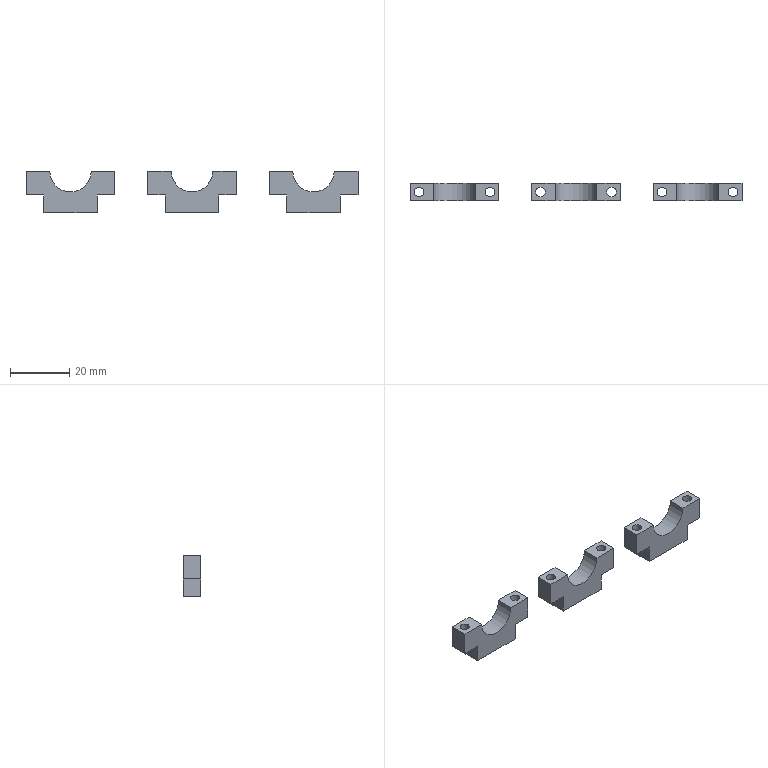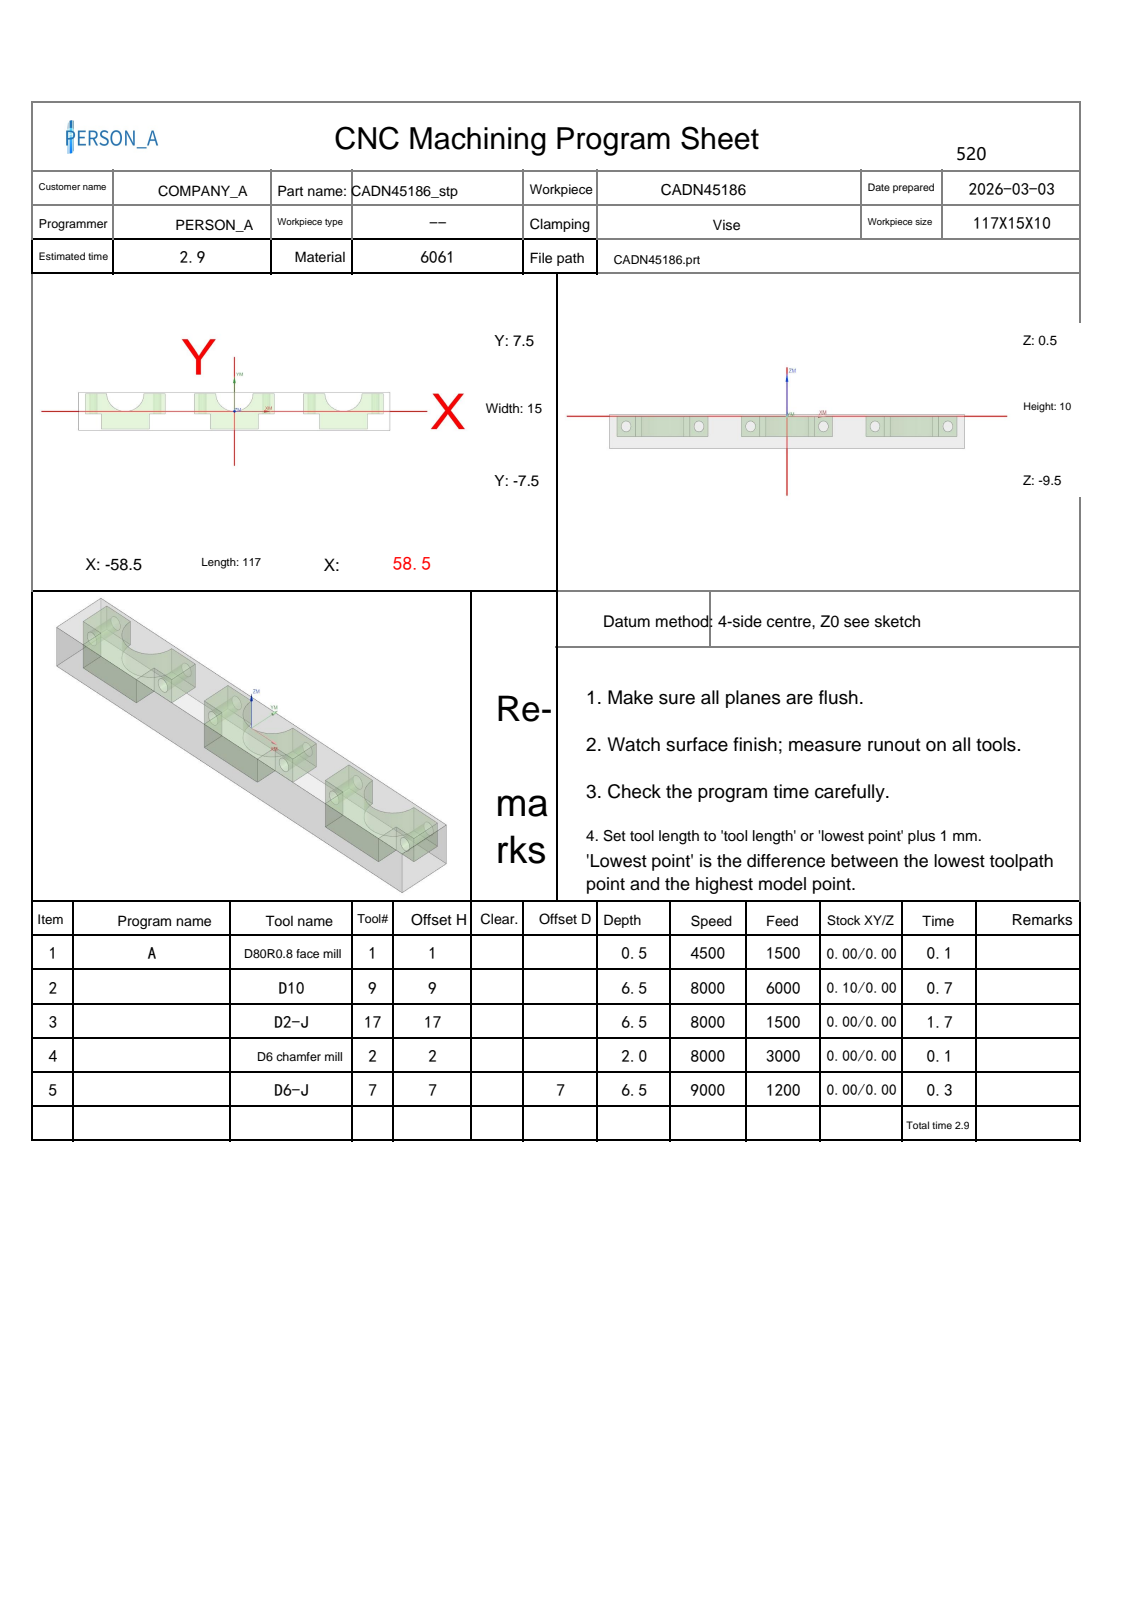NC program | NX | posted by the shop | part box 112 x 6 x 14 mm
Lines 1 to 633 of 5059:
%
O0001
(Machine time: 3.93 MIN)
(===Total Tool:5===)
(T1=D80R0.8 face mill D=80.  R=0.8  D-  H01 Z=0.    )
(T9=D10     D=10.  R=0.   D-  H09 Z=-6.   )
(T17=D2-J   D=2.   R=0.   D-  H17 Z=-6.   )
(T2=D6 chamfer mill   D=6.   R=0.   D-  H02 Z=-1.5  )
(T7=D6-J    D=6.   R=0.   D7  H07 Z=-6.   )
G80 G90 G17 G49 G40
G91 G28 Z0
M01
N1 T01 M06
(D80R0.8 face mill  D=80. R=0.8 H=01 ce=0.00 di=0.00)
(MAX_Z=50. MIN_Z=0. Time=0.15M)
G00 G90 G54 X101. Y0.0 M03 S4500
G43 H01 Z50.
M08
Z2.
G01 Z0.0 F1500.
X96.
X-96.
X-101.
Z2.
G00 Z50.
G91 G28 Z0.0
M05
M09
G91 G28 Z0.0
M01
N2 T09 M06
(D10  D=10. R=0. H=09 ce=0.10 di=0.00)
(MAX_Z=50. MIN_Z=-6. Time=0.65M)
G00 G90 G54 X41. Y-12.1 M03 S8000
G43 H09 Z50.
M08
Z.5
G01 X32. Z.447 F6000.
G02 X26.9 Y-7. Z.401 I0.0 J5.1
G01 Y-6.1 Z.395
X26. Z.39
G02 X20.9 Y-1. Z.343 I0.0 J5.1
G01 Y7. Z.297
G02 X26. Y12.1 Z.25 I5.1 J0.0
G01 X34. Z.203
G02 X39.1 Y7. Z.156 I0.0 J-5.1
G03 X41. Y5.1 Z.139 I1.9 J0.0
X42.9 Y7. Z.121 I0.0 J1.9
G02 X48. Y12.1 Z.075 I5.1 J0.0
G01 X56. Z.028
G02 X61.1 Y7. Z-.019 I0.0 J-5.1
G01 Y-1. Z-.066
G02 X56. Y-6.1 Z-.112 I-5.1 J0.0
G01 X55.1 Z-.118
Y-7. Z-.123
G02 X50. Y-12.1 Z-.17 I-5.1 J0.0
G01 X32. Z-.275
G02 X26.9 Y-7. Z-.322 I0.0 J5.1
G01 Y-6.1 Z-.327
X26. Z-.332
G02 X20.9 Y-1. Z-.379 I0.0 J5.1
G01 Y7. Z-.426
G02 X26. Y12.1 Z-.472 I5.1 J0.0
G01 X34. Z-.519
G02 X39.1 Y7. Z-.566 I0.0 J-5.1
G03 X41. Y5.1 Z-.583 I1.9 J0.0
X42.9 Y7. Z-.601 I0.0 J1.9
G02 X48. Y12.1 Z-.648 I5.1 J0.0
G01 X56. Z-.694
G02 X61.1 Y7. Z-.741 I0.0 J-5.1
G01 Y-1. Z-.788
G02 X56. Y-6.1 Z-.835 I-5.1 J0.0
G01 X55.1 Z-.84
Y-7. Z-.845
G02 X50. Y-12.1 Z-.892 I-5.1 J0.0
G01 X32. Z-.997
G02 X26.9 Y-7. Z-1.044 I0.0 J5.1
G01 Y-6.1 Z-1.049
X26. Z-1.054
G02 X20.9 Y-1. Z-1.101 I0.0 J5.1
G01 Y7. Z-1.148
G02 X26. Y12.1 Z-1.195 I5.1 J0.0
G01 X34. Z-1.241
G02 X39.1 Y7. Z-1.288 I0.0 J-5.1
G03 X41. Y5.1 Z-1.306 I1.9 J0.0
X42.9 Y7. Z-1.323 I0.0 J1.9
G02 X48. Y12.1 Z-1.37 I5.1 J0.0
G01 X56. Z-1.417
G02 X61.1 Y7. Z-1.463 I0.0 J-5.1
G01 Y-1. Z-1.51
G02 X56. Y-6.1 Z-1.557 I-5.1 J0.0
G01 X55.1 Z-1.562
Y-7. Z-1.567
G02 X50. Y-12.1 Z-1.614 I-5.1 J0.0
G01 X32. Z-1.719
G02 X26.9 Y-7. Z-1.766 I0.0 J5.1
G01 Y-6.1 Z-1.771
X26. Z-1.777
G02 X20.9 Y-1. Z-1.823 I0.0 J5.1
G01 Y7. Z-1.87
G02 X26. Y12.1 Z-1.917 I5.1 J0.0
G01 X34. Z-1.964
G02 X39.1 Y7. Z-2.01 I0.0 J-5.1
G03 X41. Y5.1 Z-2.028 I1.9 J0.0
X42.9 Y7. Z-2.045 I0.0 J1.9
G02 X48. Y12.1 Z-2.092 I5.1 J0.0
G01 X56. Z-2.139
G02 X61.1 Y7. Z-2.186 I0.0 J-5.1
G01 Y-1. Z-2.232
G02 X56. Y-6.1 Z-2.279 I-5.1 J0.0
G01 X55.1 Z-2.284
Y-7. Z-2.29
G02 X50. Y-12.1 Z-2.336 I-5.1 J0.0
G01 X32. Z-2.441
G02 X26.9 Y-7. Z-2.488 I0.0 J5.1
G01 Y-6.1 Z-2.493
X26. Z-2.499
G02 X20.9 Y-1. Z-2.546 I0.0 J5.1
G01 Y7. Z-2.592
G02 X26. Y12.1 Z-2.639 I5.1 J0.0
G01 X34. Z-2.686
G02 X39.1 Y7. Z-2.733 I0.0 J-5.1
G03 X41. Y5.1 Z-2.75 I1.9 J0.0
X42.9 Y7. Z-2.767 I0.0 J1.9
G02 X48. Y12.1 Z-2.814 I5.1 J0.0
G01 X56. Z-2.861
G02 X61.1 Y7. Z-2.908 I0.0 J-5.1
G01 Y-1. Z-2.954
G02 X56. Y-6.1 Z-3.001 I-5.1 J0.0
G01 X55.1 Z-3.007
Y-7. Z-3.012
G02 X50. Y-12.1 Z-3.059 I-5.1 J0.0
G01 X32. Z-3.164
G02 X26.9 Y-7. Z-3.21 I0.0 J5.1
G01 Y-6.1 Z-3.216
X26. Z-3.221
G02 X20.9 Y-1. Z-3.268 I0.0 J5.1
G01 Y7. Z-3.314
G02 X26. Y12.1 Z-3.361 I5.1 J0.0
G01 X34. Z-3.408
G02 X39.1 Y7. Z-3.455 I0.0 J-5.1
G03 X41. Y5.1 Z-3.472 I1.9 J0.0
X42.9 Y7. Z-3.49 I0.0 J1.9
G02 X48. Y12.1 Z-3.536 I5.1 J0.0
G01 X56. Z-3.583
G02 X61.1 Y7. Z-3.63 I0.0 J-5.1
G01 Y-1. Z-3.677
G02 X56. Y-6.1 Z-3.723 I-5.1 J0.0
G01 X55.1 Z-3.729
Y-7. Z-3.734
G02 X50. Y-12.1 Z-3.781 I-5.1 J0.0
G01 X32. Z-3.886
G02 X26.9 Y-7. Z-3.933 I0.0 J5.1
G01 Y-6.1 Z-3.938
X26. Z-3.943
G02 X20.9 Y-1. Z-3.99 I0.0 J5.1
G01 Y7. Z-4.037
G02 X26. Y12.1 Z-4.084 I5.1 J0.0
G01 X34. Z-4.13
G02 X39.1 Y7. Z-4.177 I0.0 J-5.1
G03 X41. Y5.1 Z-4.194 I1.9 J0.0
X42.9 Y7. Z-4.212 I0.0 J1.9
G02 X48. Y12.1 Z-4.259 I5.1 J0.0
G01 X56. Z-4.305
G02 X61.1 Y7. Z-4.352 I0.0 J-5.1
G01 Y-1. Z-4.399
G02 X56. Y-6.1 Z-4.446 I-5.1 J0.0
G01 X55.1 Z-4.451
Y-7. Z-4.456
G02 X50. Y-12.1 Z-4.503 I-5.1 J0.0
G01 X32. Z-4.608
G02 X26.9 Y-7. Z-4.655 I0.0 J5.1
G01 Y-6.1 Z-4.66
X26. Z-4.665
G02 X20.9 Y-1. Z-4.712 I0.0 J5.1
G01 Y7. Z-4.759
G02 X26. Y12.1 Z-4.806 I5.1 J0.0
G01 X34. Z-4.852
G02 X39.1 Y7. Z-4.899 I0.0 J-5.1
G03 X41. Y5.1 Z-4.917 I1.9 J0.0
X42.9 Y7. Z-4.934 I0.0 J1.9
G02 X48. Y12.1 Z-4.981 I5.1 J0.0
G01 X56. Z-5.028
G02 X61.1 Y7. Z-5.074 I0.0 J-5.1
G01 Y-1. Z-5.121
G02 X56. Y-6.1 Z-5.168 I-5.1 J0.0
G01 X55.1 Z-5.173
Y-7. Z-5.178
G02 X50. Y-12.1 Z-5.225 I-5.1 J0.0
G01 X32. Z-5.33
G02 X26.9 Y-7. Z-5.377 I0.0 J5.1
G01 Y-6.1 Z-5.382
X26. Z-5.388
G02 X20.9 Y-1. Z-5.434 I0.0 J5.1
G01 Y7. Z-5.481
G02 X26. Y12.1 Z-5.528 I5.1 J0.0
G01 X34. Z-5.575
G02 X39.1 Y7. Z-5.621 I0.0 J-5.1
G03 X41. Y5.1 Z-5.639 I1.9 J0.0
X42.9 Y7. Z-5.656 I0.0 J1.9
G02 X48. Y12.1 Z-5.703 I5.1 J0.0
G01 X56. Z-5.75
G02 X61.1 Y7. Z-5.797 I0.0 J-5.1
G01 Y-1. Z-5.843
G02 X56. Y-6.1 Z-5.89 I-5.1 J0.0
G01 X55.1 Z-5.895
Y-7. Z-5.901
G02 X50. Y-12.1 Z-5.947 I-5.1 J0.0
G01 X41. Z-6.
X32.
G02 X26.9 Y-7. I0.0 J5.1
G01 Y-6.1
X26.
G02 X20.9 Y-1. I0.0 J5.1
G01 Y7.
G02 X26. Y12.1 I5.1 J0.0
G01 X34.
G02 X39.1 Y7. I0.0 J-5.1
G03 X41. Y5.1 I1.9 J0.0
X42.9 Y7. I0.0 J1.9
G02 X48. Y12.1 I5.1 J0.0
G01 X56.
G02 X61.1 Y7. I0.0 J-5.1
G01 Y-1.
G02 X56. Y-6.1 I-5.1 J0.0
G01 X55.1
Y-7.
G02 X50. Y-12.1 I-5.1 J0.0
G01 X41.
X40.5
Z-5.
G00 Z50.
X0.0
Z.5
G01 X-9. Z.447
G02 X-14.1 Y-7. Z.401 I0.0 J5.1
G01 Y-6.1 Z.395
X-15. Z.39
G02 X-20.1 Y-1. Z.343 I0.0 J5.1
G01 Y7. Z.297
G02 X-15. Y12.1 Z.25 I5.1 J0.0
G01 X-7. Z.203
G02 X-1.9 Y7. Z.156 I0.0 J-5.1
G03 X0.0 Y5.1 Z.139 I1.9 J0.0
X1.9 Y7. Z.121 I0.0 J1.9
G02 X7. Y12.1 Z.075 I5.1 J0.0
G01 X15. Z.028
G02 X20.1 Y7. Z-.019 I0.0 J-5.1
G01 Y-1. Z-.066
G02 X15. Y-6.1 Z-.112 I-5.1 J0.0
G01 X14.1 Z-.118
Y-7. Z-.123
G02 X9. Y-12.1 Z-.17 I-5.1 J0.0
G01 X-9. Z-.275
G02 X-14.1 Y-7. Z-.322 I0.0 J5.1
G01 Y-6.1 Z-.327
X-15. Z-.332
G02 X-20.1 Y-1. Z-.379 I0.0 J5.1
G01 Y7. Z-.426
G02 X-15. Y12.1 Z-.472 I5.1 J0.0
G01 X-7. Z-.519
G02 X-1.9 Y7. Z-.566 I0.0 J-5.1
G03 X0.0 Y5.1 Z-.583 I1.9 J0.0
X1.9 Y7. Z-.601 I0.0 J1.9
G02 X7. Y12.1 Z-.648 I5.1 J0.0
G01 X15. Z-.694
G02 X20.1 Y7. Z-.741 I0.0 J-5.1
G01 Y-1. Z-.788
G02 X15. Y-6.1 Z-.835 I-5.1 J0.0
G01 X14.1 Z-.84
Y-7. Z-.845
G02 X9. Y-12.1 Z-.892 I-5.1 J0.0
G01 X-9. Z-.997
G02 X-14.1 Y-7. Z-1.044 I0.0 J5.1
G01 Y-6.1 Z-1.049
X-15. Z-1.054
G02 X-20.1 Y-1. Z-1.101 I0.0 J5.1
G01 Y7. Z-1.148
G02 X-15. Y12.1 Z-1.195 I5.1 J0.0
G01 X-7. Z-1.241
G02 X-1.9 Y7. Z-1.288 I0.0 J-5.1
G03 X0.0 Y5.1 Z-1.306 I1.9 J0.0
X1.9 Y7. Z-1.323 I0.0 J1.9
G02 X7. Y12.1 Z-1.37 I5.1 J0.0
G01 X15. Z-1.417
G02 X20.1 Y7. Z-1.463 I0.0 J-5.1
G01 Y-1. Z-1.51
G02 X15. Y-6.1 Z-1.557 I-5.1 J0.0
G01 X14.1 Z-1.562
Y-7. Z-1.567
G02 X9. Y-12.1 Z-1.614 I-5.1 J0.0
G01 X-9. Z-1.719
G02 X-14.1 Y-7. Z-1.766 I0.0 J5.1
G01 Y-6.1 Z-1.771
X-15. Z-1.777
G02 X-20.1 Y-1. Z-1.823 I0.0 J5.1
G01 Y7. Z-1.87
G02 X-15. Y12.1 Z-1.917 I5.1 J0.0
G01 X-7. Z-1.964
G02 X-1.9 Y7. Z-2.01 I0.0 J-5.1
G03 X0.0 Y5.1 Z-2.028 I1.9 J0.0
X1.9 Y7. Z-2.045 I0.0 J1.9
G02 X7. Y12.1 Z-2.092 I5.1 J0.0
G01 X15. Z-2.139
G02 X20.1 Y7. Z-2.186 I0.0 J-5.1
G01 Y-1. Z-2.232
G02 X15. Y-6.1 Z-2.279 I-5.1 J0.0
G01 X14.1 Z-2.284
Y-7. Z-2.29
G02 X9. Y-12.1 Z-2.336 I-5.1 J0.0
G01 X-9. Z-2.441
G02 X-14.1 Y-7. Z-2.488 I0.0 J5.1
G01 Y-6.1 Z-2.493
X-15. Z-2.499
G02 X-20.1 Y-1. Z-2.546 I0.0 J5.1
G01 Y7. Z-2.592
G02 X-15. Y12.1 Z-2.639 I5.1 J0.0
G01 X-7. Z-2.686
G02 X-1.9 Y7. Z-2.733 I0.0 J-5.1
G03 X0.0 Y5.1 Z-2.75 I1.9 J0.0
X1.9 Y7. Z-2.767 I0.0 J1.9
G02 X7. Y12.1 Z-2.814 I5.1 J0.0
G01 X15. Z-2.861
G02 X20.1 Y7. Z-2.908 I0.0 J-5.1
G01 Y-1. Z-2.954
G02 X15. Y-6.1 Z-3.001 I-5.1 J0.0
G01 X14.1 Z-3.007
Y-7. Z-3.012
G02 X9. Y-12.1 Z-3.059 I-5.1 J0.0
G01 X-9. Z-3.164
G02 X-14.1 Y-7. Z-3.21 I0.0 J5.1
G01 Y-6.1 Z-3.216
X-15. Z-3.221
G02 X-20.1 Y-1. Z-3.268 I0.0 J5.1
G01 Y7. Z-3.314
G02 X-15. Y12.1 Z-3.361 I5.1 J0.0
G01 X-7. Z-3.408
G02 X-1.9 Y7. Z-3.455 I0.0 J-5.1
G03 X0.0 Y5.1 Z-3.472 I1.9 J0.0
X1.9 Y7. Z-3.49 I0.0 J1.9
G02 X7. Y12.1 Z-3.536 I5.1 J0.0
G01 X15. Z-3.583
G02 X20.1 Y7. Z-3.63 I0.0 J-5.1
G01 Y-1. Z-3.677
G02 X15. Y-6.1 Z-3.723 I-5.1 J0.0
G01 X14.1 Z-3.729
Y-7. Z-3.734
G02 X9. Y-12.1 Z-3.781 I-5.1 J0.0
G01 X-9. Z-3.886
G02 X-14.1 Y-7. Z-3.933 I0.0 J5.1
G01 Y-6.1 Z-3.938
X-15. Z-3.943
G02 X-20.1 Y-1. Z-3.99 I0.0 J5.1
G01 Y7. Z-4.037
G02 X-15. Y12.1 Z-4.084 I5.1 J0.0
G01 X-7. Z-4.13
G02 X-1.9 Y7. Z-4.177 I0.0 J-5.1
G03 X0.0 Y5.1 Z-4.194 I1.9 J0.0
X1.9 Y7. Z-4.212 I0.0 J1.9
G02 X7. Y12.1 Z-4.259 I5.1 J0.0
G01 X15. Z-4.305
G02 X20.1 Y7. Z-4.352 I0.0 J-5.1
G01 Y-1. Z-4.399
G02 X15. Y-6.1 Z-4.446 I-5.1 J0.0
G01 X14.1 Z-4.451
Y-7. Z-4.456
G02 X9. Y-12.1 Z-4.503 I-5.1 J0.0
G01 X-9. Z-4.608
G02 X-14.1 Y-7. Z-4.655 I0.0 J5.1
G01 Y-6.1 Z-4.66
X-15. Z-4.665
G02 X-20.1 Y-1. Z-4.712 I0.0 J5.1
G01 Y7. Z-4.759
G02 X-15. Y12.1 Z-4.806 I5.1 J0.0
G01 X-7. Z-4.852
G02 X-1.9 Y7. Z-4.899 I0.0 J-5.1
G03 X0.0 Y5.1 Z-4.917 I1.9 J0.0
X1.9 Y7. Z-4.934 I0.0 J1.9
G02 X7. Y12.1 Z-4.981 I5.1 J0.0
G01 X15. Z-5.028
G02 X20.1 Y7. Z-5.074 I0.0 J-5.1
G01 Y-1. Z-5.121
G02 X15. Y-6.1 Z-5.168 I-5.1 J0.0
G01 X14.1 Z-5.173
Y-7. Z-5.178
G02 X9. Y-12.1 Z-5.225 I-5.1 J0.0
G01 X-9. Z-5.33
G02 X-14.1 Y-7. Z-5.377 I0.0 J5.1
G01 Y-6.1 Z-5.382
X-15. Z-5.388
G02 X-20.1 Y-1. Z-5.434 I0.0 J5.1
G01 Y7. Z-5.481
G02 X-15. Y12.1 Z-5.528 I5.1 J0.0
G01 X-7. Z-5.575
G02 X-1.9 Y7. Z-5.621 I0.0 J-5.1
G03 X0.0 Y5.1 Z-5.639 I1.9 J0.0
X1.9 Y7. Z-5.656 I0.0 J1.9
G02 X7. Y12.1 Z-5.703 I5.1 J0.0
G01 X15. Z-5.75
G02 X20.1 Y7. Z-5.797 I0.0 J-5.1
G01 Y-1. Z-5.843
G02 X15. Y-6.1 Z-5.89 I-5.1 J0.0
G01 X14.1 Z-5.895
Y-7. Z-5.901
G02 X9. Y-12.1 Z-5.947 I-5.1 J0.0
G01 X0.0 Z-6.
X-9.
G02 X-14.1 Y-7. I0.0 J5.1
G01 Y-6.1
X-15.
G02 X-20.1 Y-1. I0.0 J5.1
G01 Y7.
G02 X-15. Y12.1 I5.1 J0.0
G01 X-7.
G02 X-1.9 Y7. I0.0 J-5.1
G03 X0.0 Y5.1 I1.9 J0.0
X1.9 Y7. I0.0 J1.9
G02 X7. Y12.1 I5.1 J0.0
G01 X15.
G02 X20.1 Y7. I0.0 J-5.1
G01 Y-1.
G02 X15. Y-6.1 I-5.1 J0.0
G01 X14.1
Y-7.
G02 X9. Y-12.1 I-5.1 J0.0
G01 X0.0
X-.5
Z-5.
G00 Z50.
X-41.
Z.5
G01 X-50. Z.447
G02 X-55.1 Y-7. Z.401 I0.0 J5.1
G01 Y-6.1 Z.395
X-56. Z.39
G02 X-61.1 Y-1. Z.343 I0.0 J5.1
G01 Y7. Z.297
G02 X-56. Y12.1 Z.25 I5.1 J0.0
G01 X-48. Z.203
G02 X-42.9 Y7. Z.156 I0.0 J-5.1
G03 X-41. Y5.1 Z.139 I1.9 J0.0
X-39.1 Y7. Z.121 I0.0 J1.9
G02 X-34. Y12.1 Z.075 I5.1 J0.0
G01 X-26. Z.028
G02 X-20.9 Y7. Z-.019 I0.0 J-5.1
G01 Y-1. Z-.066
G02 X-26. Y-6.1 Z-.112 I-5.1 J0.0
G01 X-26.9 Z-.118
Y-7. Z-.123
G02 X-32. Y-12.1 Z-.17 I-5.1 J0.0
G01 X-50. Z-.275
G02 X-55.1 Y-7. Z-.322 I0.0 J5.1
G01 Y-6.1 Z-.327
X-56. Z-.332
G02 X-61.1 Y-1. Z-.379 I0.0 J5.1
G01 Y7. Z-.426
G02 X-56. Y12.1 Z-.472 I5.1 J0.0
G01 X-48. Z-.519
G02 X-42.9 Y7. Z-.566 I0.0 J-5.1
G03 X-41. Y5.1 Z-.583 I1.9 J0.0
X-39.1 Y7. Z-.601 I0.0 J1.9
G02 X-34. Y12.1 Z-.648 I5.1 J0.0
G01 X-26. Z-.694
G02 X-20.9 Y7. Z-.741 I0.0 J-5.1
G01 Y-1. Z-.788
G02 X-26. Y-6.1 Z-.835 I-5.1 J0.0
G01 X-26.9 Z-.84
Y-7. Z-.845
G02 X-32. Y-12.1 Z-.892 I-5.1 J0.0
G01 X-50. Z-.997
G02 X-55.1 Y-7. Z-1.044 I0.0 J5.1
G01 Y-6.1 Z-1.049
X-56. Z-1.054
G02 X-61.1 Y-1. Z-1.101 I0.0 J5.1
G01 Y7. Z-1.148
G02 X-56. Y12.1 Z-1.195 I5.1 J0.0
G01 X-48. Z-1.241
G02 X-42.9 Y7. Z-1.288 I0.0 J-5.1
G03 X-41. Y5.1 Z-1.306 I1.9 J0.0
X-39.1 Y7. Z-1.323 I0.0 J1.9
G02 X-34. Y12.1 Z-1.37 I5.1 J0.0
G01 X-26. Z-1.417
G02 X-20.9 Y7. Z-1.463 I0.0 J-5.1
G01 Y-1. Z-1.51
G02 X-26. Y-6.1 Z-1.557 I-5.1 J0.0
G01 X-26.9 Z-1.562
Y-7. Z-1.567
G02 X-32. Y-12.1 Z-1.614 I-5.1 J0.0
G01 X-50. Z-1.719
G02 X-55.1 Y-7. Z-1.766 I0.0 J5.1
G01 Y-6.1 Z-1.771
X-56. Z-1.777
G02 X-61.1 Y-1. Z-1.823 I0.0 J5.1
G01 Y7. Z-1.87
G02 X-56. Y12.1 Z-1.917 I5.1 J0.0
G01 X-48. Z-1.964
G02 X-42.9 Y7. Z-2.01 I0.0 J-5.1
G03 X-41. Y5.1 Z-2.028 I1.9 J0.0
X-39.1 Y7. Z-2.045 I0.0 J1.9
G02 X-34. Y12.1 Z-2.092 I5.1 J0.0
G01 X-26. Z-2.139
G02 X-20.9 Y7. Z-2.186 I0.0 J-5.1
G01 Y-1. Z-2.232
G02 X-26. Y-6.1 Z-2.279 I-5.1 J0.0
G01 X-26.9 Z-2.284
Y-7. Z-2.29
G02 X-32. Y-12.1 Z-2.336 I-5.1 J0.0
G01 X-50. Z-2.441
G02 X-55.1 Y-7. Z-2.488 I0.0 J5.1
G01 Y-6.1 Z-2.493
X-56. Z-2.499
G02 X-61.1 Y-1. Z-2.546 I0.0 J5.1
G01 Y7. Z-2.592
G02 X-56. Y12.1 Z-2.639 I5.1 J0.0
G01 X-48. Z-2.686
G02 X-42.9 Y7. Z-2.733 I0.0 J-5.1
G03 X-41. Y5.1 Z-2.75 I1.9 J0.0
X-39.1 Y7. Z-2.767 I0.0 J1.9
G02 X-34. Y12.1 Z-2.814 I5.1 J0.0
G01 X-26. Z-2.861
G02 X-20.9 Y7. Z-2.908 I0.0 J-5.1
G01 Y-1. Z-2.954
G02 X-26. Y-6.1 Z-3.001 I-5.1 J0.0
G01 X-26.9 Z-3.007
Y-7. Z-3.012
G02 X-32. Y-12.1 Z-3.059 I-5.1 J0.0
G01 X-50. Z-3.164
G02 X-55.1 Y-7. Z-3.21 I0.0 J5.1
G01 Y-6.1 Z-3.216
X-56. Z-3.221
G02 X-61.1 Y-1. Z-3.268 I0.0 J5.1
G01 Y7. Z-3.314
G02 X-56. Y12.1 Z-3.361 I5.1 J0.0
G01 X-48. Z-3.408
G02 X-42.9 Y7. Z-3.455 I0.0 J-5.1
G03 X-41. Y5.1 Z-3.472 I1.9 J0.0
X-39.1 Y7. Z-3.49 I0.0 J1.9
G02 X-34. Y12.1 Z-3.536 I5.1 J0.0
G01 X-26. Z-3.583
G02 X-20.9 Y7. Z-3.63 I0.0 J-5.1
G01 Y-1. Z-3.677
G02 X-26. Y-6.1 Z-3.723 I-5.1 J0.0
G01 X-26.9 Z-3.729
Y-7. Z-3.734
G02 X-32. Y-12.1 Z-3.781 I-5.1 J0.0
G01 X-50. Z-3.886
G02 X-55.1 Y-7. Z-3.933 I0.0 J5.1
G01 Y-6.1 Z-3.938
X-56. Z-3.943
G02 X-61.1 Y-1. Z-3.99 I0.0 J5.1
G01 Y7. Z-4.037
G02 X-56. Y12.1 Z-4.084 I5.1 J0.0
G01 X-48. Z-4.13
G02 X-42.9 Y7. Z-4.177 I0.0 J-5.1
G03 X-41. Y5.1 Z-4.194 I1.9 J0.0
X-39.1 Y7. Z-4.212 I0.0 J1.9
G02 X-34. Y12.1 Z-4.259 I5.1 J0.0
G01 X-26. Z-4.305
G02 X-20.9 Y7. Z-4.352 I0.0 J-5.1
G01 Y-1. Z-4.399
G02 X-26. Y-6.1 Z-4.446 I-5.1 J0.0
G01 X-26.9 Z-4.451
Y-7. Z-4.456
G02 X-32. Y-12.1 Z-4.503 I-5.1 J0.0
G01 X-50. Z-4.608
G02 X-55.1 Y-7. Z-4.655 I0.0 J5.1
G01 Y-6.1 Z-4.66
X-56. Z-4.665
G02 X-61.1 Y-1. Z-4.712 I0.0 J5.1
G01 Y7. Z-4.759
G02 X-56. Y12.1 Z-4.806 I5.1 J0.0
G01 X-48. Z-4.852
G02 X-42.9 Y7. Z-4.899 I0.0 J-5.1
G03 X-41. Y5.1 Z-4.917 I1.9 J0.0
X-39.1 Y7. Z-4.934 I0.0 J1.9
G02 X-34. Y12.1 Z-4.981 I5.1 J0.0
G01 X-26. Z-5.028
G02 X-20.9 Y7. Z-5.074 I0.0 J-5.1
G01 Y-1. Z-5.121
G02 X-26. Y-6.1 Z-5.168 I-5.1 J0.0
G01 X-26.9 Z-5.173
Y-7. Z-5.178
G02 X-32. Y-12.1 Z-5.225 I-5.1 J0.0
G01 X-50. Z-5.33
G02 X-55.1 Y-7. Z-5.377 I0.0 J5.1
G01 Y-6.1 Z-5.382
X-56. Z-5.388
G02 X-61.1 Y-1. Z-5.434 I0.0 J5.1
G01 Y7. Z-5.481
G02 X-56. Y12.1 Z-5.528 I5.1 J0.0
G01 X-48. Z-5.575
G02 X-42.9 Y7. Z-5.621 I0.0 J-5.1
G03 X-41. Y5.1 Z-5.639 I1.9 J0.0
X-39.1 Y7. Z-5.656 I0.0 J1.9
G02 X-34. Y12.1 Z-5.703 I5.1 J0.0
G01 X-26. Z-5.75
G02 X-20.9 Y7. Z-5.797 I0.0 J-5.1
G01 Y-1. Z-5.843
G02 X-26. Y-6.1 Z-5.89 I-5.1 J0.0
G01 X-26.9 Z-5.895
Y-7. Z-5.901
G02 X-32. Y-12.1 Z-5.947 I-5.1 J0.0
G01 X-41. Z-6.
X-50.
G02 X-55.1 Y-7. I0.0 J5.1
G01 Y-6.1
X-56.
G02 X-61.1 Y-1. I0.0 J5.1
G01 Y7.
G02 X-56. Y12.1 I5.1 J0.0
G01 X-48.
G02 X-42.9 Y7. I0.0 J-5.1
G03 X-41. Y5.1 I1.9 J0.0
X-39.1 Y7. I0.0 J1.9
G02 X-34. Y12.1 I5.1 J0.0
G01 X-26.
G02 X-20.9 Y7. I0.0 J-5.1
G01 Y-1.
G02 X-26. Y-6.1 I-5.1 J0.0
G01 X-26.9
Y-7.
G02 X-32. Y-12.1 I-5.1 J0.0
G01 X-41.
X-41.5
Z-5.
G00 Z50.
G91 G28 Z0.0
M05
M09
G91 G28 Z0.0
M01